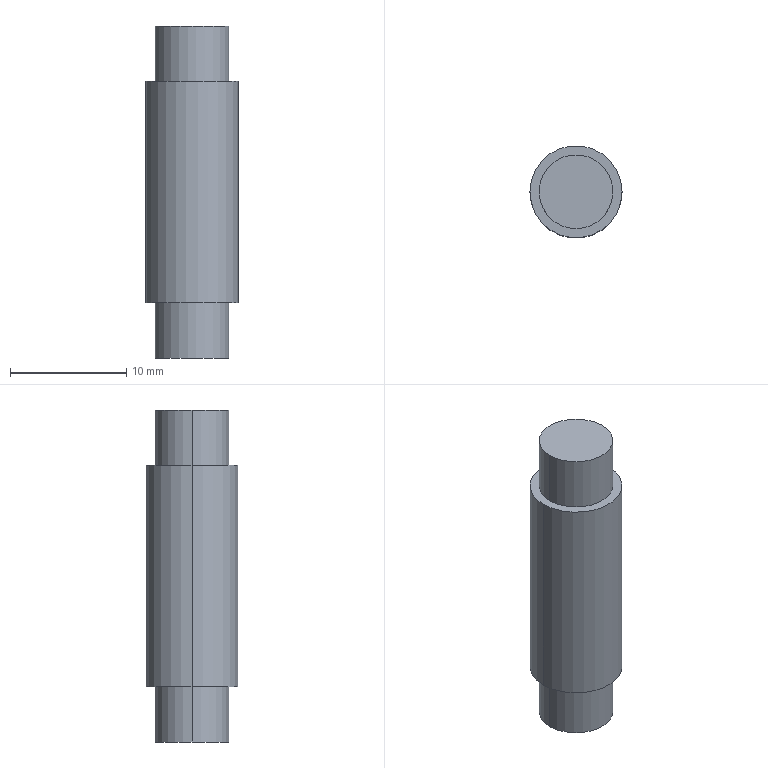Part | SolidWorks | features Extrusion 1, ICE 1 | 1 solid | 10 faces | box 7.925 x 7.925 x 28.575 mm | volume 1241 mm3 | cylinder 6 | plane 4 | commonest cylinder face diameters 6.35 x4 7.925 x2
STEP:
#1=CARTESIAN_POINT('',(3.175,0.,-14.287));
#2=VERTEX_POINT('',#1);
#3=CARTESIAN_POINT('',(-3.175,0.,-14.287));
#4=VERTEX_POINT('',#3);
#5=CARTESIAN_POINT('',(0.,0.,-14.287));
#6=DIRECTION('',(0.,0.,1.));
#7=DIRECTION('',(1.,0.,0.));
#8=AXIS2_PLACEMENT_3D('',#5,#6,#7);
#9=CIRCLE('',#8,3.175);
#10=EDGE_CURVE('',#2,#4,#9,.T.);
#11=ORIENTED_EDGE('',*,*,#10,.T.);
#12=CARTESIAN_POINT('',(-3.175,0.,-9.525));
#13=VERTEX_POINT('',#12);
#14=CARTESIAN_POINT('',(-3.175,0.,-14.287));
#15=DIRECTION('',(0.,0.,1.));
#16=VECTOR('',#15,1000.);
#17=LINE('',#14,#16);
#18=EDGE_CURVE('',#4,#13,#17,.T.);
#19=ORIENTED_EDGE('',*,*,#18,.T.);
#20=CARTESIAN_POINT('',(3.175,0.,-9.525));
#21=VERTEX_POINT('',#20);
#22=CARTESIAN_POINT('',(0.,0.,-9.525));
#23=DIRECTION('',(0.,0.,1.));
#24=DIRECTION('',(1.,0.,0.));
#25=AXIS2_PLACEMENT_3D('',#22,#23,#24);
#26=CIRCLE('',#25,3.175);
#27=EDGE_CURVE('',#21,#13,#26,.T.);
#28=ORIENTED_EDGE('',*,*,#27,.F.);
#29=CARTESIAN_POINT('',(3.175,0.,-14.287));
#30=DIRECTION('',(0.,0.,1.));
#31=VECTOR('',#30,1000.);
#32=LINE('',#29,#31);
#33=EDGE_CURVE('',#2,#21,#32,.T.);
#34=ORIENTED_EDGE('',*,*,#33,.F.);
#35=EDGE_LOOP('',(#11,#19,#28,#34));
#36=FACE_OUTER_BOUND('',#35,.T.);
#37=CARTESIAN_POINT('',(0.,0.,-14.287));
#38=DIRECTION('',(0.,0.,1.));
#39=DIRECTION('',(1.,0.,0.));
#40=AXIS2_PLACEMENT_3D('',#37,#38,#39);
#41=CYLINDRICAL_SURFACE('',#40,3.175);
#42=ADVANCED_FACE('',(#36),#41,.T.);
#43=CARTESIAN_POINT('',(3.175,0.,9.525));
#44=VERTEX_POINT('',#43);
#45=CARTESIAN_POINT('',(-3.175,0.,9.525));
#46=VERTEX_POINT('',#45);
#47=CARTESIAN_POINT('',(0.,0.,9.525));
#48=DIRECTION('',(0.,0.,1.));
#49=DIRECTION('',(1.,0.,0.));
#50=AXIS2_PLACEMENT_3D('',#47,#48,#49);
#51=CIRCLE('',#50,3.175);
#52=EDGE_CURVE('',#44,#46,#51,.T.);
#53=ORIENTED_EDGE('',*,*,#52,.T.);
#54=CARTESIAN_POINT('',(-3.175,0.,14.287));
#55=VERTEX_POINT('',#54);
#56=CARTESIAN_POINT('',(-3.175,0.,-14.287));
#57=DIRECTION('',(0.,0.,1.));
#58=VECTOR('',#57,1000.);
#59=LINE('',#56,#58);
#60=EDGE_CURVE('',#46,#55,#59,.T.);
#61=ORIENTED_EDGE('',*,*,#60,.T.);
#62=CARTESIAN_POINT('',(3.175,0.,14.287));
#63=VERTEX_POINT('',#62);
#64=CARTESIAN_POINT('',(0.,0.,14.287));
#65=DIRECTION('',(0.,0.,1.));
#66=DIRECTION('',(1.,0.,0.));
#67=AXIS2_PLACEMENT_3D('',#64,#65,#66);
#68=CIRCLE('',#67,3.175);
#69=EDGE_CURVE('',#63,#55,#68,.T.);
#70=ORIENTED_EDGE('',*,*,#69,.F.);
#71=CARTESIAN_POINT('',(3.175,0.,-14.287));
#72=DIRECTION('',(0.,0.,1.));
#73=VECTOR('',#72,1000.);
#74=LINE('',#71,#73);
#75=EDGE_CURVE('',#44,#63,#74,.T.);
#76=ORIENTED_EDGE('',*,*,#75,.F.);
#77=EDGE_LOOP('',(#53,#61,#70,#76));
#78=FACE_OUTER_BOUND('',#77,.T.);
#79=CARTESIAN_POINT('',(0.,0.,-14.287));
#80=DIRECTION('',(0.,0.,1.));
#81=DIRECTION('',(1.,0.,0.));
#82=AXIS2_PLACEMENT_3D('',#79,#80,#81);
#83=CYLINDRICAL_SURFACE('',#82,3.175);
#84=ADVANCED_FACE('',(#78),#83,.T.);
#85=CARTESIAN_POINT('',(3.962,0.,-9.525));
#86=VERTEX_POINT('',#85);
#87=CARTESIAN_POINT('',(-3.962,0.,-9.525));
#88=VERTEX_POINT('',#87);
#89=CARTESIAN_POINT('',(0.,0.,-9.525));
#90=DIRECTION('',(0.,0.,1.));
#91=DIRECTION('',(1.,0.,0.));
#92=AXIS2_PLACEMENT_3D('',#89,#90,#91);
#93=CIRCLE('',#92,3.962);
#94=EDGE_CURVE('',#86,#88,#93,.T.);
#95=ORIENTED_EDGE('',*,*,#94,.T.);
#96=CARTESIAN_POINT('',(-3.962,0.,9.525));
#97=VERTEX_POINT('',#96);
#98=CARTESIAN_POINT('',(-3.962,0.,-9.525));
#99=DIRECTION('',(0.,0.,1.));
#100=VECTOR('',#99,1000.);
#101=LINE('',#98,#100);
#102=EDGE_CURVE('',#88,#97,#101,.T.);
#103=ORIENTED_EDGE('',*,*,#102,.T.);
#104=CARTESIAN_POINT('',(3.962,0.,9.525));
#105=VERTEX_POINT('',#104);
#106=CARTESIAN_POINT('',(0.,0.,9.525));
#107=DIRECTION('',(0.,0.,1.));
#108=DIRECTION('',(1.,0.,0.));
#109=AXIS2_PLACEMENT_3D('',#106,#107,#108);
#110=CIRCLE('',#109,3.962);
#111=EDGE_CURVE('',#105,#97,#110,.T.);
#112=ORIENTED_EDGE('',*,*,#111,.F.);
#113=CARTESIAN_POINT('',(3.962,0.,-9.525));
#114=DIRECTION('',(0.,0.,1.));
#115=VECTOR('',#114,1000.);
#116=LINE('',#113,#115);
#117=EDGE_CURVE('',#86,#105,#116,.T.);
#118=ORIENTED_EDGE('',*,*,#117,.F.);
#119=EDGE_LOOP('',(#95,#103,#112,#118));
#120=FACE_OUTER_BOUND('',#119,.T.);
#121=CARTESIAN_POINT('',(0.,0.,-9.525));
#122=DIRECTION('',(0.,0.,1.));
#123=DIRECTION('',(1.,0.,0.));
#124=AXIS2_PLACEMENT_3D('',#121,#122,#123);
#125=CYLINDRICAL_SURFACE('',#124,3.962);
#126=ADVANCED_FACE('',(#120),#125,.T.);
#127=ORIENTED_EDGE('',*,*,#102,.F.);
#128=CARTESIAN_POINT('',(0.,0.,-9.525));
#129=DIRECTION('',(0.,0.,1.));
#130=DIRECTION('',(1.,0.,0.));
#131=AXIS2_PLACEMENT_3D('',#128,#129,#130);
#132=CIRCLE('',#131,3.962);
#133=EDGE_CURVE('',#88,#86,#132,.T.);
#134=ORIENTED_EDGE('',*,*,#133,.T.);
#135=ORIENTED_EDGE('',*,*,#117,.T.);
#136=CARTESIAN_POINT('',(0.,0.,9.525));
#137=DIRECTION('',(0.,0.,1.));
#138=DIRECTION('',(1.,0.,0.));
#139=AXIS2_PLACEMENT_3D('',#136,#137,#138);
#140=CIRCLE('',#139,3.962);
#141=EDGE_CURVE('',#97,#105,#140,.T.);
#142=ORIENTED_EDGE('',*,*,#141,.F.);
#143=EDGE_LOOP('',(#127,#134,#135,#142));
#144=FACE_OUTER_BOUND('',#143,.T.);
#145=CARTESIAN_POINT('',(0.,0.,-9.525));
#146=DIRECTION('',(0.,0.,1.));
#147=DIRECTION('',(1.,0.,0.));
#148=AXIS2_PLACEMENT_3D('',#145,#146,#147);
#149=CYLINDRICAL_SURFACE('',#148,3.962);
#150=ADVANCED_FACE('',(#144),#149,.T.);
#151=ORIENTED_EDGE('',*,*,#27,.T.);
#152=CARTESIAN_POINT('',(0.,0.,-9.525));
#153=DIRECTION('',(0.,0.,1.));
#154=DIRECTION('',(1.,0.,0.));
#155=AXIS2_PLACEMENT_3D('',#152,#153,#154);
#156=CIRCLE('',#155,3.175);
#157=EDGE_CURVE('',#13,#21,#156,.T.);
#158=ORIENTED_EDGE('',*,*,#157,.T.);
#159=EDGE_LOOP('',(#151,#158));
#160=FACE_BOUND('',#159,.T.);
#161=ORIENTED_EDGE('',*,*,#94,.F.);
#162=ORIENTED_EDGE('',*,*,#133,.F.);
#163=EDGE_LOOP('',(#161,#162));
#164=FACE_OUTER_BOUND('',#163,.T.);
#165=CARTESIAN_POINT('',(0.,0.,-9.525));
#166=DIRECTION('',(0.,0.,1.));
#167=DIRECTION('',(1.,0.,0.));
#168=AXIS2_PLACEMENT_3D('',#165,#166,#167);
#169=PLANE('',#168);
#170=ADVANCED_FACE('',(#160,#164),#169,.F.);
#171=ORIENTED_EDGE('',*,*,#52,.F.);
#172=CARTESIAN_POINT('',(0.,0.,9.525));
#173=DIRECTION('',(0.,0.,1.));
#174=DIRECTION('',(1.,0.,0.));
#175=AXIS2_PLACEMENT_3D('',#172,#173,#174);
#176=CIRCLE('',#175,3.175);
#177=EDGE_CURVE('',#46,#44,#176,.T.);
#178=ORIENTED_EDGE('',*,*,#177,.F.);
#179=EDGE_LOOP('',(#171,#178));
#180=FACE_BOUND('',#179,.T.);
#181=ORIENTED_EDGE('',*,*,#111,.T.);
#182=ORIENTED_EDGE('',*,*,#141,.T.);
#183=EDGE_LOOP('',(#181,#182));
#184=FACE_OUTER_BOUND('',#183,.T.);
#185=CARTESIAN_POINT('',(0.,0.,9.525));
#186=DIRECTION('',(0.,0.,1.));
#187=DIRECTION('',(1.,0.,0.));
#188=AXIS2_PLACEMENT_3D('',#185,#186,#187);
#189=PLANE('',#188);
#190=ADVANCED_FACE('',(#180,#184),#189,.T.);
#191=ORIENTED_EDGE('',*,*,#69,.T.);
#192=CARTESIAN_POINT('',(0.,0.,14.287));
#193=DIRECTION('',(0.,0.,1.));
#194=DIRECTION('',(1.,0.,0.));
#195=AXIS2_PLACEMENT_3D('',#192,#193,#194);
#196=CIRCLE('',#195,3.175);
#197=EDGE_CURVE('',#55,#63,#196,.T.);
#198=ORIENTED_EDGE('',*,*,#197,.T.);
#199=EDGE_LOOP('',(#191,#198));
#200=FACE_OUTER_BOUND('',#199,.T.);
#201=CARTESIAN_POINT('',(0.,0.,14.287));
#202=DIRECTION('',(0.,0.,1.));
#203=DIRECTION('',(1.,0.,0.));
#204=AXIS2_PLACEMENT_3D('',#201,#202,#203);
#205=PLANE('',#204);
#206=ADVANCED_FACE('',(#200),#205,.T.);
#207=ORIENTED_EDGE('',*,*,#60,.F.);
#208=ORIENTED_EDGE('',*,*,#177,.T.);
#209=ORIENTED_EDGE('',*,*,#75,.T.);
#210=ORIENTED_EDGE('',*,*,#197,.F.);
#211=EDGE_LOOP('',(#207,#208,#209,#210));
#212=FACE_OUTER_BOUND('',#211,.T.);
#213=CARTESIAN_POINT('',(0.,0.,-14.287));
#214=DIRECTION('',(0.,0.,1.));
#215=DIRECTION('',(1.,0.,0.));
#216=AXIS2_PLACEMENT_3D('',#213,#214,#215);
#217=CYLINDRICAL_SURFACE('',#216,3.175);
#218=ADVANCED_FACE('',(#212),#217,.T.);
#219=ORIENTED_EDGE('',*,*,#18,.F.);
#220=CARTESIAN_POINT('',(0.,0.,-14.287));
#221=DIRECTION('',(0.,0.,1.));
#222=DIRECTION('',(1.,0.,0.));
#223=AXIS2_PLACEMENT_3D('',#220,#221,#222);
#224=CIRCLE('',#223,3.175);
#225=EDGE_CURVE('',#4,#2,#224,.T.);
#226=ORIENTED_EDGE('',*,*,#225,.T.);
#227=ORIENTED_EDGE('',*,*,#33,.T.);
#228=ORIENTED_EDGE('',*,*,#157,.F.);
#229=EDGE_LOOP('',(#219,#226,#227,#228));
#230=FACE_OUTER_BOUND('',#229,.T.);
#231=CARTESIAN_POINT('',(0.,0.,-14.287));
#232=DIRECTION('',(0.,0.,1.));
#233=DIRECTION('',(1.,0.,0.));
#234=AXIS2_PLACEMENT_3D('',#231,#232,#233);
#235=CYLINDRICAL_SURFACE('',#234,3.175);
#236=ADVANCED_FACE('',(#230),#235,.T.);
#237=ORIENTED_EDGE('',*,*,#10,.F.);
#238=ORIENTED_EDGE('',*,*,#225,.F.);
#239=EDGE_LOOP('',(#237,#238));
#240=FACE_OUTER_BOUND('',#239,.T.);
#241=CARTESIAN_POINT('',(0.,0.,-14.287));
#242=DIRECTION('',(0.,0.,1.));
#243=DIRECTION('',(1.,0.,0.));
#244=AXIS2_PLACEMENT_3D('',#241,#242,#243);
#245=PLANE('',#244);
#246=ADVANCED_FACE('',(#240),#245,.F.);
#247=CLOSED_SHELL('',(#42,#84,#126,#150,#170,#190,#206,#218,#236,#246));
#248=MANIFOLD_SOLID_BREP('',#247);
#249=CARTESIAN_POINT('',(0.,0.,0.));
#250=DIRECTION('',(0.,0.,1.));
#251=DIRECTION('',(1.,0.,0.));
#252=AXIS2_PLACEMENT_3D('',#249,#250,#251);
#253=(LENGTH_UNIT()NAMED_UNIT(*)SI_UNIT(.MILLI.,.METRE.));
#254=UNCERTAINTY_MEASURE_WITH_UNIT(LENGTH_MEASURE(0.00001),#253,'','');
#255=(NAMED_UNIT(*)PLANE_ANGLE_UNIT()SI_UNIT($,.RADIAN.));
#256=(NAMED_UNIT(*)SI_UNIT($,.STERADIAN.)SOLID_ANGLE_UNIT());
#257=(GEOMETRIC_REPRESENTATION_CONTEXT(3)GLOBAL_UNCERTAINTY_ASSIGNED_CONTEXT((#254))GLOBAL_UNIT_ASSIGNED_CONTEXT((#253,#255,#256))REPRESENTATION_CONTEXT('',''));
#258=ADVANCED_BREP_SHAPE_REPRESENTATION('',(#248,#252),#257);